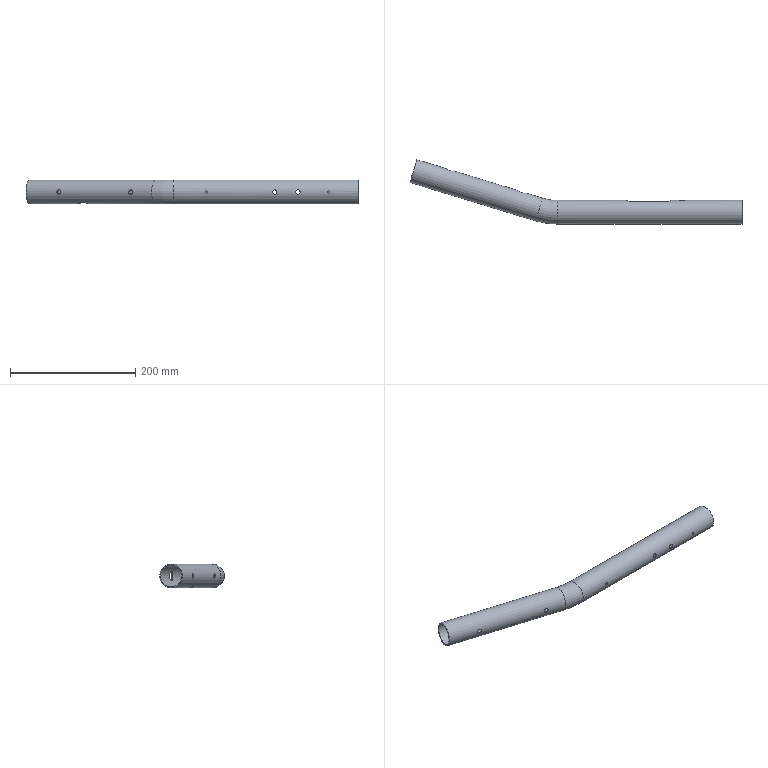Part | STEP file | PN_0002 | 1 solid | 22 faces | box 530.631 x 103.035 x 38.1 mm | volume 88866 mm3 | cylinder 16 | plane 4 | torus 2 | commonest cylinder face diameters 7 x4 3.5 x2 15 x2 18 x2 35.1 x2 38.1 x2